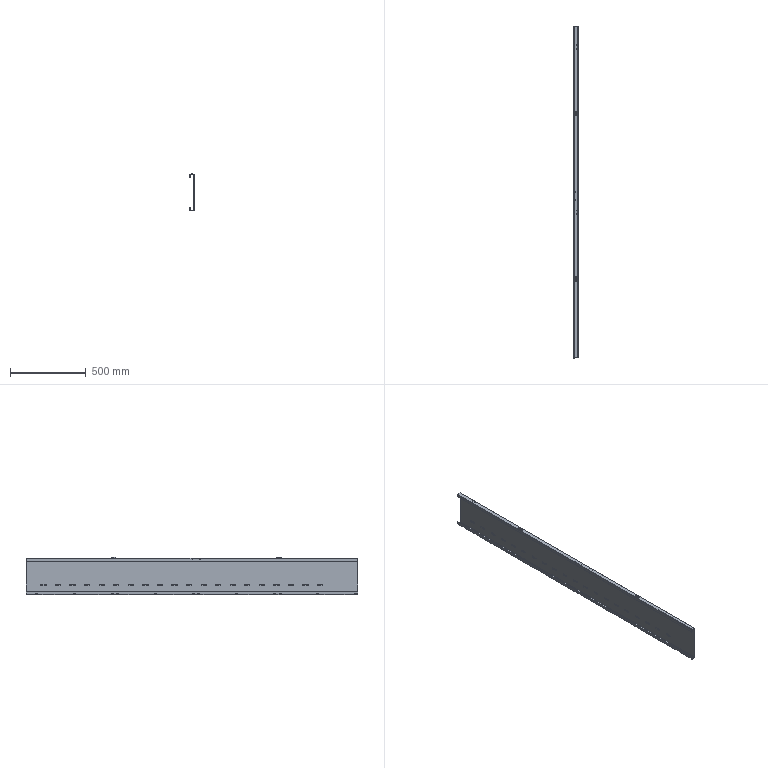Part | NX | features solid 2 | 1 solid | 908 faces | box 28.183 x 2189 x 244 mm | volume 1386395 mm3 | plane 714 | cylinder 194 | commonest cylinder face diameters 4 x86 1.86 x38 5.86 x38 11.1 x32